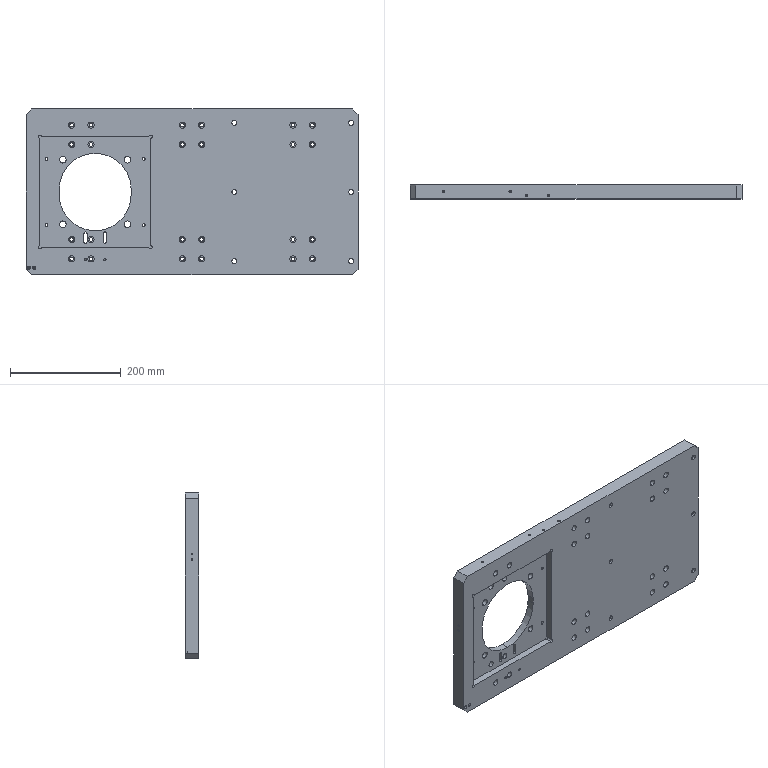Part | SolidWorks | features HoleWzd 11, Cut 2, Chamfer 1, Extrusion 1 | 1 solid | 244 faces | box 600 x 25 x 300 mm | volume 3745145 mm3 | cylinder 175 | plane 53 | cone 16 | commonest cylinder face diameters 6.6 x48 11 x48 4.2 x12 9 x12 15 x12 6 x10